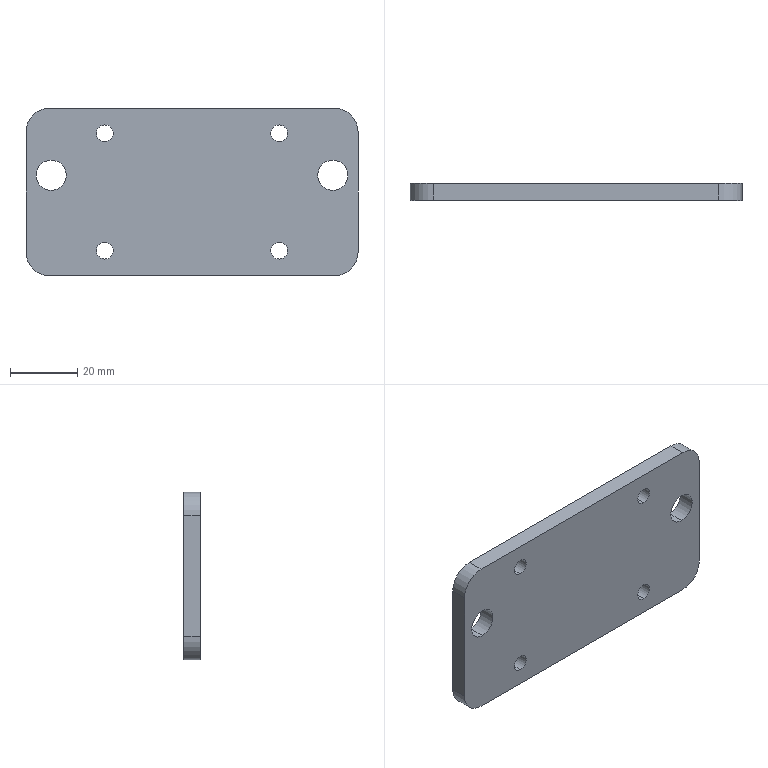Part | STEP file | 1.6米脚轮垫块 | 1 solid | 22 faces | box 99 x 5 x 50 mm | volume 23511 mm3 | cylinder 16 | plane 6 | commonest cylinder face diameters 5 x8 9 x4 14 x4
STEP:
#1=CARTESIAN_POINT('',(91.5,5.,-15.5));
#2=VERTEX_POINT('',#1);
#3=CARTESIAN_POINT('',(91.5,5.,-24.5));
#4=VERTEX_POINT('',#3);
#5=CARTESIAN_POINT('',(91.5,5.,-20.));
#6=DIRECTION('',(0.,-1.,0.));
#7=DIRECTION('',(0.,0.,-1.));
#8=AXIS2_PLACEMENT_3D('',#5,#6,#7);
#9=CIRCLE('',#8,4.5);
#10=EDGE_CURVE('',#2,#4,#9,.T.);
#11=ORIENTED_EDGE('',*,*,#10,.F.);
#12=CARTESIAN_POINT('',(91.5,0.,-15.5));
#13=VERTEX_POINT('',#12);
#14=CARTESIAN_POINT('',(91.5,10.,-15.5));
#15=DIRECTION('',(0.,-1.,0.));
#16=VECTOR('',#15,1000.);
#17=LINE('',#14,#16);
#18=EDGE_CURVE('',#2,#13,#17,.T.);
#19=ORIENTED_EDGE('',*,*,#18,.T.);
#20=CARTESIAN_POINT('',(91.5,0.,-24.5));
#21=VERTEX_POINT('',#20);
#22=CARTESIAN_POINT('',(91.5,0.,-20.));
#23=DIRECTION('',(0.,-1.,0.));
#24=DIRECTION('',(0.,0.,-1.));
#25=AXIS2_PLACEMENT_3D('',#22,#23,#24);
#26=CIRCLE('',#25,4.5);
#27=EDGE_CURVE('',#13,#21,#26,.T.);
#28=ORIENTED_EDGE('',*,*,#27,.T.);
#29=CARTESIAN_POINT('',(91.5,10.,-24.5));
#30=DIRECTION('',(0.,-1.,0.));
#31=VECTOR('',#30,1000.);
#32=LINE('',#29,#31);
#33=EDGE_CURVE('',#4,#21,#32,.T.);
#34=ORIENTED_EDGE('',*,*,#33,.F.);
#35=EDGE_LOOP('',(#11,#19,#28,#34));
#36=FACE_OUTER_BOUND('',#35,.T.);
#37=CARTESIAN_POINT('',(91.5,10.,-20.));
#38=DIRECTION('',(0.,-1.,0.));
#39=DIRECTION('',(0.,0.,-1.));
#40=AXIS2_PLACEMENT_3D('',#37,#38,#39);
#41=CYLINDRICAL_SURFACE('',#40,4.5);
#42=ADVANCED_FACE('',(#36),#41,.F.);
#43=CARTESIAN_POINT('',(7.5,5.,-15.5));
#44=VERTEX_POINT('',#43);
#45=CARTESIAN_POINT('',(7.5,5.,-24.5));
#46=VERTEX_POINT('',#45);
#47=CARTESIAN_POINT('',(7.5,5.,-20.));
#48=DIRECTION('',(0.,-1.,0.));
#49=DIRECTION('',(0.,0.,-1.));
#50=AXIS2_PLACEMENT_3D('',#47,#48,#49);
#51=CIRCLE('',#50,4.5);
#52=EDGE_CURVE('',#44,#46,#51,.T.);
#53=ORIENTED_EDGE('',*,*,#52,.F.);
#54=CARTESIAN_POINT('',(7.5,0.,-15.5));
#55=VERTEX_POINT('',#54);
#56=CARTESIAN_POINT('',(7.5,10.,-15.5));
#57=DIRECTION('',(0.,-1.,0.));
#58=VECTOR('',#57,1000.);
#59=LINE('',#56,#58);
#60=EDGE_CURVE('',#44,#55,#59,.T.);
#61=ORIENTED_EDGE('',*,*,#60,.T.);
#62=CARTESIAN_POINT('',(7.5,0.,-24.5));
#63=VERTEX_POINT('',#62);
#64=CARTESIAN_POINT('',(7.5,0.,-20.));
#65=DIRECTION('',(0.,-1.,0.));
#66=DIRECTION('',(0.,0.,-1.));
#67=AXIS2_PLACEMENT_3D('',#64,#65,#66);
#68=CIRCLE('',#67,4.5);
#69=EDGE_CURVE('',#55,#63,#68,.T.);
#70=ORIENTED_EDGE('',*,*,#69,.T.);
#71=CARTESIAN_POINT('',(7.5,10.,-24.5));
#72=DIRECTION('',(0.,-1.,0.));
#73=VECTOR('',#72,1000.);
#74=LINE('',#71,#73);
#75=EDGE_CURVE('',#46,#63,#74,.T.);
#76=ORIENTED_EDGE('',*,*,#75,.F.);
#77=EDGE_LOOP('',(#53,#61,#70,#76));
#78=FACE_OUTER_BOUND('',#77,.T.);
#79=CARTESIAN_POINT('',(7.5,10.,-20.));
#80=DIRECTION('',(0.,-1.,0.));
#81=DIRECTION('',(0.,0.,-1.));
#82=AXIS2_PLACEMENT_3D('',#79,#80,#81);
#83=CYLINDRICAL_SURFACE('',#82,4.5);
#84=ADVANCED_FACE('',(#78),#83,.F.);
#85=CARTESIAN_POINT('',(75.5,5.,-40.));
#86=VERTEX_POINT('',#85);
#87=CARTESIAN_POINT('',(75.5,5.,-45.));
#88=VERTEX_POINT('',#87);
#89=CARTESIAN_POINT('',(75.5,5.,-42.5));
#90=DIRECTION('',(0.,-1.,0.));
#91=DIRECTION('',(0.,0.,-1.));
#92=AXIS2_PLACEMENT_3D('',#89,#90,#91);
#93=CIRCLE('',#92,2.5);
#94=EDGE_CURVE('',#86,#88,#93,.T.);
#95=ORIENTED_EDGE('',*,*,#94,.F.);
#96=CARTESIAN_POINT('',(75.5,0.,-40.));
#97=VERTEX_POINT('',#96);
#98=CARTESIAN_POINT('',(75.5,0.,-40.));
#99=DIRECTION('',(0.,-1.,0.));
#100=VECTOR('',#99,1000.);
#101=LINE('',#98,#100);
#102=EDGE_CURVE('',#86,#97,#101,.T.);
#103=ORIENTED_EDGE('',*,*,#102,.T.);
#104=CARTESIAN_POINT('',(75.5,0.,-45.));
#105=VERTEX_POINT('',#104);
#106=CARTESIAN_POINT('',(75.5,0.,-42.5));
#107=DIRECTION('',(0.,-1.,0.));
#108=DIRECTION('',(0.,0.,-1.));
#109=AXIS2_PLACEMENT_3D('',#106,#107,#108);
#110=CIRCLE('',#109,2.5);
#111=EDGE_CURVE('',#97,#105,#110,.T.);
#112=ORIENTED_EDGE('',*,*,#111,.T.);
#113=CARTESIAN_POINT('',(75.5,0.,-45.));
#114=DIRECTION('',(0.,-1.,0.));
#115=VECTOR('',#114,1000.);
#116=LINE('',#113,#115);
#117=EDGE_CURVE('',#88,#105,#116,.T.);
#118=ORIENTED_EDGE('',*,*,#117,.F.);
#119=EDGE_LOOP('',(#95,#103,#112,#118));
#120=FACE_OUTER_BOUND('',#119,.T.);
#121=CARTESIAN_POINT('',(75.5,0.,-42.5));
#122=DIRECTION('',(0.,-1.,0.));
#123=DIRECTION('',(0.,0.,-1.));
#124=AXIS2_PLACEMENT_3D('',#121,#122,#123);
#125=CYLINDRICAL_SURFACE('',#124,2.5);
#126=ADVANCED_FACE('',(#120),#125,.F.);
#127=CARTESIAN_POINT('',(23.5,5.,-40.));
#128=VERTEX_POINT('',#127);
#129=CARTESIAN_POINT('',(23.5,5.,-45.));
#130=VERTEX_POINT('',#129);
#131=CARTESIAN_POINT('',(23.5,5.,-42.5));
#132=DIRECTION('',(0.,-1.,0.));
#133=DIRECTION('',(0.,0.,-1.));
#134=AXIS2_PLACEMENT_3D('',#131,#132,#133);
#135=CIRCLE('',#134,2.5);
#136=EDGE_CURVE('',#128,#130,#135,.T.);
#137=ORIENTED_EDGE('',*,*,#136,.F.);
#138=CARTESIAN_POINT('',(23.5,0.,-40.));
#139=VERTEX_POINT('',#138);
#140=CARTESIAN_POINT('',(23.5,0.,-40.));
#141=DIRECTION('',(0.,-1.,0.));
#142=VECTOR('',#141,1000.);
#143=LINE('',#140,#142);
#144=EDGE_CURVE('',#128,#139,#143,.T.);
#145=ORIENTED_EDGE('',*,*,#144,.T.);
#146=CARTESIAN_POINT('',(23.5,0.,-45.));
#147=VERTEX_POINT('',#146);
#148=CARTESIAN_POINT('',(23.5,0.,-42.5));
#149=DIRECTION('',(0.,-1.,0.));
#150=DIRECTION('',(0.,0.,-1.));
#151=AXIS2_PLACEMENT_3D('',#148,#149,#150);
#152=CIRCLE('',#151,2.5);
#153=EDGE_CURVE('',#139,#147,#152,.T.);
#154=ORIENTED_EDGE('',*,*,#153,.T.);
#155=CARTESIAN_POINT('',(23.5,0.,-45.));
#156=DIRECTION('',(0.,-1.,0.));
#157=VECTOR('',#156,1000.);
#158=LINE('',#155,#157);
#159=EDGE_CURVE('',#130,#147,#158,.T.);
#160=ORIENTED_EDGE('',*,*,#159,.F.);
#161=EDGE_LOOP('',(#137,#145,#154,#160));
#162=FACE_OUTER_BOUND('',#161,.T.);
#163=CARTESIAN_POINT('',(23.5,0.,-42.5));
#164=DIRECTION('',(0.,-1.,0.));
#165=DIRECTION('',(0.,0.,-1.));
#166=AXIS2_PLACEMENT_3D('',#163,#164,#165);
#167=CYLINDRICAL_SURFACE('',#166,2.5);
#168=ADVANCED_FACE('',(#162),#167,.F.);
#169=CARTESIAN_POINT('',(75.5,5.,-5.));
#170=VERTEX_POINT('',#169);
#171=CARTESIAN_POINT('',(75.5,5.,-10.));
#172=VERTEX_POINT('',#171);
#173=CARTESIAN_POINT('',(75.5,5.,-7.5));
#174=DIRECTION('',(0.,-1.,0.));
#175=DIRECTION('',(0.,0.,-1.));
#176=AXIS2_PLACEMENT_3D('',#173,#174,#175);
#177=CIRCLE('',#176,2.5);
#178=EDGE_CURVE('',#170,#172,#177,.T.);
#179=ORIENTED_EDGE('',*,*,#178,.F.);
#180=CARTESIAN_POINT('',(75.5,0.,-5.));
#181=VERTEX_POINT('',#180);
#182=CARTESIAN_POINT('',(75.5,0.,-5.));
#183=DIRECTION('',(0.,-1.,0.));
#184=VECTOR('',#183,1000.);
#185=LINE('',#182,#184);
#186=EDGE_CURVE('',#170,#181,#185,.T.);
#187=ORIENTED_EDGE('',*,*,#186,.T.);
#188=CARTESIAN_POINT('',(75.5,0.,-10.));
#189=VERTEX_POINT('',#188);
#190=CARTESIAN_POINT('',(75.5,0.,-7.5));
#191=DIRECTION('',(0.,-1.,0.));
#192=DIRECTION('',(0.,0.,-1.));
#193=AXIS2_PLACEMENT_3D('',#190,#191,#192);
#194=CIRCLE('',#193,2.5);
#195=EDGE_CURVE('',#181,#189,#194,.T.);
#196=ORIENTED_EDGE('',*,*,#195,.T.);
#197=CARTESIAN_POINT('',(75.5,0.,-10.));
#198=DIRECTION('',(0.,-1.,0.));
#199=VECTOR('',#198,1000.);
#200=LINE('',#197,#199);
#201=EDGE_CURVE('',#172,#189,#200,.T.);
#202=ORIENTED_EDGE('',*,*,#201,.F.);
#203=EDGE_LOOP('',(#179,#187,#196,#202));
#204=FACE_OUTER_BOUND('',#203,.T.);
#205=CARTESIAN_POINT('',(75.5,0.,-7.5));
#206=DIRECTION('',(0.,-1.,0.));
#207=DIRECTION('',(0.,0.,-1.));
#208=AXIS2_PLACEMENT_3D('',#205,#206,#207);
#209=CYLINDRICAL_SURFACE('',#208,2.5);
#210=ADVANCED_FACE('',(#204),#209,.F.);
#211=CARTESIAN_POINT('',(23.5,5.,-5.));
#212=VERTEX_POINT('',#211);
#213=CARTESIAN_POINT('',(23.5,5.,-10.));
#214=VERTEX_POINT('',#213);
#215=CARTESIAN_POINT('',(23.5,5.,-7.5));
#216=DIRECTION('',(0.,-1.,0.));
#217=DIRECTION('',(0.,0.,-1.));
#218=AXIS2_PLACEMENT_3D('',#215,#216,#217);
#219=CIRCLE('',#218,2.5);
#220=EDGE_CURVE('',#212,#214,#219,.T.);
#221=ORIENTED_EDGE('',*,*,#220,.F.);
#222=CARTESIAN_POINT('',(23.5,0.,-5.));
#223=VERTEX_POINT('',#222);
#224=CARTESIAN_POINT('',(23.5,0.,-5.));
#225=DIRECTION('',(0.,-1.,0.));
#226=VECTOR('',#225,1000.);
#227=LINE('',#224,#226);
#228=EDGE_CURVE('',#212,#223,#227,.T.);
#229=ORIENTED_EDGE('',*,*,#228,.T.);
#230=CARTESIAN_POINT('',(23.5,0.,-10.));
#231=VERTEX_POINT('',#230);
#232=CARTESIAN_POINT('',(23.5,0.,-7.5));
#233=DIRECTION('',(0.,-1.,0.));
#234=DIRECTION('',(0.,0.,-1.));
#235=AXIS2_PLACEMENT_3D('',#232,#233,#234);
#236=CIRCLE('',#235,2.5);
#237=EDGE_CURVE('',#223,#231,#236,.T.);
#238=ORIENTED_EDGE('',*,*,#237,.T.);
#239=CARTESIAN_POINT('',(23.5,0.,-10.));
#240=DIRECTION('',(0.,-1.,0.));
#241=VECTOR('',#240,1000.);
#242=LINE('',#239,#241);
#243=EDGE_CURVE('',#214,#231,#242,.T.);
#244=ORIENTED_EDGE('',*,*,#243,.F.);
#245=EDGE_LOOP('',(#221,#229,#238,#244));
#246=FACE_OUTER_BOUND('',#245,.T.);
#247=CARTESIAN_POINT('',(23.5,0.,-7.5));
#248=DIRECTION('',(0.,-1.,0.));
#249=DIRECTION('',(0.,0.,-1.));
#250=AXIS2_PLACEMENT_3D('',#247,#248,#249);
#251=CYLINDRICAL_SURFACE('',#250,2.5);
#252=ADVANCED_FACE('',(#246),#251,.F.);
#253=CARTESIAN_POINT('',(0.,5.,-43.));
#254=VERTEX_POINT('',#253);
#255=CARTESIAN_POINT('',(0.,5.,-7.));
#256=VERTEX_POINT('',#255);
#257=CARTESIAN_POINT('',(0.,5.,0.));
#258=DIRECTION('',(0.,0.,1.));
#259=VECTOR('',#258,1000.);
#260=LINE('',#257,#259);
#261=EDGE_CURVE('',#254,#256,#260,.T.);
#262=ORIENTED_EDGE('',*,*,#261,.F.);
#263=CARTESIAN_POINT('',(0.,0.,-43.));
#264=VERTEX_POINT('',#263);
#265=CARTESIAN_POINT('',(0.,5.,-43.));
#266=DIRECTION('',(0.,-1.,0.));
#267=VECTOR('',#266,1000.);
#268=LINE('',#265,#267);
#269=EDGE_CURVE('',#254,#264,#268,.T.);
#270=ORIENTED_EDGE('',*,*,#269,.T.);
#271=CARTESIAN_POINT('',(0.,0.,-7.));
#272=VERTEX_POINT('',#271);
#273=CARTESIAN_POINT('',(0.,0.,0.));
#274=DIRECTION('',(0.,0.,1.));
#275=VECTOR('',#274,1000.);
#276=LINE('',#273,#275);
#277=EDGE_CURVE('',#264,#272,#276,.T.);
#278=ORIENTED_EDGE('',*,*,#277,.T.);
#279=CARTESIAN_POINT('',(0.,5.,-7.));
#280=DIRECTION('',(0.,1.,0.));
#281=VECTOR('',#280,1000.);
#282=LINE('',#279,#281);
#283=EDGE_CURVE('',#272,#256,#282,.T.);
#284=ORIENTED_EDGE('',*,*,#283,.T.);
#285=EDGE_LOOP('',(#262,#270,#278,#284));
#286=FACE_OUTER_BOUND('',#285,.T.);
#287=CARTESIAN_POINT('',(0.,5.,0.));
#288=DIRECTION('',(1.,0.,0.));
#289=DIRECTION('',(0.,0.,-1.));
#290=AXIS2_PLACEMENT_3D('',#287,#288,#289);
#291=PLANE('',#290);
#292=ADVANCED_FACE('',(#286),#291,.F.);
#293=CARTESIAN_POINT('',(7.,0.,0.));
#294=VERTEX_POINT('',#293);
#295=CARTESIAN_POINT('',(92.,0.,0.));
#296=VERTEX_POINT('',#295);
#297=CARTESIAN_POINT('',(0.,0.,0.));
#298=DIRECTION('',(1.,0.,0.));
#299=VECTOR('',#298,1000.);
#300=LINE('',#297,#299);
#301=EDGE_CURVE('',#294,#296,#300,.T.);
#302=ORIENTED_EDGE('',*,*,#301,.T.);
#303=CARTESIAN_POINT('',(92.,5.,0.));
#304=VERTEX_POINT('',#303);
#305=CARTESIAN_POINT('',(92.,5.,0.));
#306=DIRECTION('',(0.,1.,0.));
#307=VECTOR('',#306,1000.);
#308=LINE('',#305,#307);
#309=EDGE_CURVE('',#296,#304,#308,.T.);
#310=ORIENTED_EDGE('',*,*,#309,.T.);
#311=CARTESIAN_POINT('',(7.,5.,0.));
#312=VERTEX_POINT('',#311);
#313=CARTESIAN_POINT('',(0.,5.,0.));
#314=DIRECTION('',(1.,0.,0.));
#315=VECTOR('',#314,1000.);
#316=LINE('',#313,#315);
#317=EDGE_CURVE('',#312,#304,#316,.T.);
#318=ORIENTED_EDGE('',*,*,#317,.F.);
#319=CARTESIAN_POINT('',(7.,5.,0.));
#320=DIRECTION('',(0.,-1.,0.));
#321=VECTOR('',#320,1000.);
#322=LINE('',#319,#321);
#323=EDGE_CURVE('',#312,#294,#322,.T.);
#324=ORIENTED_EDGE('',*,*,#323,.T.);
#325=EDGE_LOOP('',(#302,#310,#318,#324));
#326=FACE_OUTER_BOUND('',#325,.T.);
#327=CARTESIAN_POINT('',(0.,5.,0.));
#328=DIRECTION('',(0.,0.,-1.));
#329=DIRECTION('',(-1.,0.,0.));
#330=AXIS2_PLACEMENT_3D('',#327,#328,#329);
#331=PLANE('',#330);
#332=ADVANCED_FACE('',(#326),#331,.F.);
#333=CARTESIAN_POINT('',(99.,0.,-7.));
#334=VERTEX_POINT('',#333);
#335=CARTESIAN_POINT('',(99.,0.,-43.));
#336=VERTEX_POINT('',#335);
#337=CARTESIAN_POINT('',(99.,0.,0.));
#338=DIRECTION('',(0.,0.,-1.));
#339=VECTOR('',#338,1000.);
#340=LINE('',#337,#339);
#341=EDGE_CURVE('',#334,#336,#340,.T.);
#342=ORIENTED_EDGE('',*,*,#341,.T.);
#343=CARTESIAN_POINT('',(99.,5.,-43.));
#344=VERTEX_POINT('',#343);
#345=CARTESIAN_POINT('',(99.,5.,-43.));
#346=DIRECTION('',(0.,1.,0.));
#347=VECTOR('',#346,1000.);
#348=LINE('',#345,#347);
#349=EDGE_CURVE('',#336,#344,#348,.T.);
#350=ORIENTED_EDGE('',*,*,#349,.T.);
#351=CARTESIAN_POINT('',(99.,5.,-7.));
#352=VERTEX_POINT('',#351);
#353=CARTESIAN_POINT('',(99.,5.,0.));
#354=DIRECTION('',(0.,0.,-1.));
#355=VECTOR('',#354,1000.);
#356=LINE('',#353,#355);
#357=EDGE_CURVE('',#352,#344,#356,.T.);
#358=ORIENTED_EDGE('',*,*,#357,.F.);
#359=CARTESIAN_POINT('',(99.,5.,-7.));
#360=DIRECTION('',(0.,-1.,0.));
#361=VECTOR('',#360,1000.);
#362=LINE('',#359,#361);
#363=EDGE_CURVE('',#352,#334,#362,.T.);
#364=ORIENTED_EDGE('',*,*,#363,.T.);
#365=EDGE_LOOP('',(#342,#350,#358,#364));
#366=FACE_OUTER_BOUND('',#365,.T.);
#367=CARTESIAN_POINT('',(99.,5.,0.));
#368=DIRECTION('',(-1.,0.,0.));
#369=DIRECTION('',(0.,0.,1.));
#370=AXIS2_PLACEMENT_3D('',#367,#368,#369);
#371=PLANE('',#370);
#372=ADVANCED_FACE('',(#366),#371,.F.);
#373=CARTESIAN_POINT('',(92.,0.,-50.));
#374=VERTEX_POINT('',#373);
#375=CARTESIAN_POINT('',(7.,0.,-50.));
#376=VERTEX_POINT('',#375);
#377=CARTESIAN_POINT('',(0.,0.,-50.));
#378=DIRECTION('',(-1.,0.,0.));
#379=VECTOR('',#378,1000.);
#380=LINE('',#377,#379);
#381=EDGE_CURVE('',#374,#376,#380,.T.);
#382=ORIENTED_EDGE('',*,*,#381,.T.);
#383=CARTESIAN_POINT('',(7.,5.,-50.));
#384=VERTEX_POINT('',#383);
#385=CARTESIAN_POINT('',(7.,5.,-50.));
#386=DIRECTION('',(0.,1.,0.));
#387=VECTOR('',#386,1000.);
#388=LINE('',#385,#387);
#389=EDGE_CURVE('',#376,#384,#388,.T.);
#390=ORIENTED_EDGE('',*,*,#389,.T.);
#391=CARTESIAN_POINT('',(92.,5.,-50.));
#392=VERTEX_POINT('',#391);
#393=CARTESIAN_POINT('',(0.,5.,-50.));
#394=DIRECTION('',(-1.,0.,0.));
#395=VECTOR('',#394,1000.);
#396=LINE('',#393,#395);
#397=EDGE_CURVE('',#392,#384,#396,.T.);
#398=ORIENTED_EDGE('',*,*,#397,.F.);
#399=CARTESIAN_POINT('',(92.,5.,-50.));
#400=DIRECTION('',(0.,-1.,0.));
#401=VECTOR('',#400,1000.);
#402=LINE('',#399,#401);
#403=EDGE_CURVE('',#392,#374,#402,.T.);
#404=ORIENTED_EDGE('',*,*,#403,.T.);
#405=EDGE_LOOP('',(#382,#390,#398,#404));
#406=FACE_OUTER_BOUND('',#405,.T.);
#407=CARTESIAN_POINT('',(0.,5.,-50.));
#408=DIRECTION('',(0.,0.,1.));
#409=DIRECTION('',(1.,0.,0.));
#410=AXIS2_PLACEMENT_3D('',#407,#408,#409);
#411=PLANE('',#410);
#412=ADVANCED_FACE('',(#406),#411,.F.);
#413=CARTESIAN_POINT('',(91.5,5.,-20.));
#414=DIRECTION('',(0.,-1.,0.));
#415=DIRECTION('',(0.,0.,-1.));
#416=AXIS2_PLACEMENT_3D('',#413,#414,#415);
#417=CIRCLE('',#416,4.5);
#418=EDGE_CURVE('',#4,#2,#417,.T.);
#419=ORIENTED_EDGE('',*,*,#418,.T.);
#420=ORIENTED_EDGE('',*,*,#10,.T.);
#421=EDGE_LOOP('',(#419,#420));
#422=FACE_BOUND('',#421,.T.);
#423=CARTESIAN_POINT('',(7.5,5.,-20.));
#424=DIRECTION('',(0.,-1.,0.));
#425=DIRECTION('',(0.,0.,-1.));
#426=AXIS2_PLACEMENT_3D('',#423,#424,#425);
#427=CIRCLE('',#426,4.5);
#428=EDGE_CURVE('',#46,#44,#427,.T.);
#429=ORIENTED_EDGE('',*,*,#428,.T.);
#430=ORIENTED_EDGE('',*,*,#52,.T.);
#431=EDGE_LOOP('',(#429,#430));
#432=FACE_BOUND('',#431,.T.);
#433=CARTESIAN_POINT('',(75.5,5.,-42.5));
#434=DIRECTION('',(0.,-1.,0.));
#435=DIRECTION('',(0.,0.,-1.));
#436=AXIS2_PLACEMENT_3D('',#433,#434,#435);
#437=CIRCLE('',#436,2.5);
#438=EDGE_CURVE('',#88,#86,#437,.T.);
#439=ORIENTED_EDGE('',*,*,#438,.T.);
#440=ORIENTED_EDGE('',*,*,#94,.T.);
#441=EDGE_LOOP('',(#439,#440));
#442=FACE_BOUND('',#441,.T.);
#443=CARTESIAN_POINT('',(23.5,5.,-42.5));
#444=DIRECTION('',(0.,-1.,0.));
#445=DIRECTION('',(0.,0.,-1.));
#446=AXIS2_PLACEMENT_3D('',#443,#444,#445);
#447=CIRCLE('',#446,2.5);
#448=EDGE_CURVE('',#130,#128,#447,.T.);
#449=ORIENTED_EDGE('',*,*,#448,.T.);
#450=ORIENTED_EDGE('',*,*,#136,.T.);
#451=EDGE_LOOP('',(#449,#450));
#452=FACE_BOUND('',#451,.T.);
#453=CARTESIAN_POINT('',(75.5,5.,-7.5));
#454=DIRECTION('',(0.,-1.,0.));
#455=DIRECTION('',(0.,0.,-1.));
#456=AXIS2_PLACEMENT_3D('',#453,#454,#455);
#457=CIRCLE('',#456,2.5);
#458=EDGE_CURVE('',#172,#170,#457,.T.);
#459=ORIENTED_EDGE('',*,*,#458,.T.);
#460=ORIENTED_EDGE('',*,*,#178,.T.);
#461=EDGE_LOOP('',(#459,#460));
#462=FACE_BOUND('',#461,.T.);
#463=CARTESIAN_POINT('',(23.5,5.,-7.5));
#464=DIRECTION('',(0.,-1.,0.));
#465=DIRECTION('',(0.,0.,-1.));
#466=AXIS2_PLACEMENT_3D('',#463,#464,#465);
#467=CIRCLE('',#466,2.5);
#468=EDGE_CURVE('',#214,#212,#467,.T.);
#469=ORIENTED_EDGE('',*,*,#468,.T.);
#470=ORIENTED_EDGE('',*,*,#220,.T.);
#471=EDGE_LOOP('',(#469,#470));
#472=FACE_BOUND('',#471,.T.);
#473=ORIENTED_EDGE('',*,*,#397,.T.);
#474=CARTESIAN_POINT('',(7.,5.,-43.));
#475=DIRECTION('',(0.,1.,0.));
#476=DIRECTION('',(0.,0.,-1.));
#477=AXIS2_PLACEMENT_3D('',#474,#475,#476);
#478=CIRCLE('',#477,7.);
#479=EDGE_CURVE('',#384,#254,#478,.T.);
#480=ORIENTED_EDGE('',*,*,#479,.T.);
#481=ORIENTED_EDGE('',*,*,#261,.T.);
#482=CARTESIAN_POINT('',(7.,5.,-7.));
#483=DIRECTION('',(0.,1.,0.));
#484=DIRECTION('',(0.,0.,-1.));
#485=AXIS2_PLACEMENT_3D('',#482,#483,#484);
#486=CIRCLE('',#485,7.);
#487=EDGE_CURVE('',#256,#312,#486,.T.);
#488=ORIENTED_EDGE('',*,*,#487,.T.);
#489=ORIENTED_EDGE('',*,*,#317,.T.);
#490=CARTESIAN_POINT('',(92.,5.,-7.));
#491=DIRECTION('',(0.,1.,0.));
#492=DIRECTION('',(0.,0.,-1.));
#493=AXIS2_PLACEMENT_3D('',#490,#491,#492);
#494=CIRCLE('',#493,7.);
#495=EDGE_CURVE('',#304,#352,#494,.T.);
#496=ORIENTED_EDGE('',*,*,#495,.T.);
#497=ORIENTED_EDGE('',*,*,#357,.T.);
#498=CARTESIAN_POINT('',(92.,5.,-43.));
#499=DIRECTION('',(0.,1.,0.));
#500=DIRECTION('',(0.,0.,-1.));
#501=AXIS2_PLACEMENT_3D('',#498,#499,#500);
#502=CIRCLE('',#501,7.);
#503=EDGE_CURVE('',#344,#392,#502,.T.);
#504=ORIENTED_EDGE('',*,*,#503,.T.);
#505=EDGE_LOOP('',(#473,#480,#481,#488,#489,#496,#497,#504));
#506=FACE_OUTER_BOUND('',#505,.T.);
#507=CARTESIAN_POINT('',(0.,5.,0.));
#508=DIRECTION('',(0.,-1.,0.));
#509=DIRECTION('',(0.,0.,-1.));
#510=AXIS2_PLACEMENT_3D('',#507,#508,#509);
#511=PLANE('',#510);
#512=ADVANCED_FACE('',(#422,#432,#442,#452,#462,#472,#506),#511,.F.);
#513=CARTESIAN_POINT('',(91.5,0.,-20.));
#514=DIRECTION('',(0.,-1.,0.));
#515=DIRECTION('',(0.,0.,-1.));
#516=AXIS2_PLACEMENT_3D('',#513,#514,#515);
#517=CIRCLE('',#516,4.5);
#518=EDGE_CURVE('',#21,#13,#517,.T.);
#519=ORIENTED_EDGE('',*,*,#518,.F.);
#520=ORIENTED_EDGE('',*,*,#27,.F.);
#521=EDGE_LOOP('',(#519,#520));
#522=FACE_BOUND('',#521,.T.);
#523=CARTESIAN_POINT('',(7.5,0.,-20.));
#524=DIRECTION('',(0.,-1.,0.));
#525=DIRECTION('',(0.,0.,-1.));
#526=AXIS2_PLACEMENT_3D('',#523,#524,#525);
#527=CIRCLE('',#526,4.5);
#528=EDGE_CURVE('',#63,#55,#527,.T.);
#529=ORIENTED_EDGE('',*,*,#528,.F.);
#530=ORIENTED_EDGE('',*,*,#69,.F.);
#531=EDGE_LOOP('',(#529,#530));
#532=FACE_BOUND('',#531,.T.);
#533=CARTESIAN_POINT('',(75.5,0.,-42.5));
#534=DIRECTION('',(0.,-1.,0.));
#535=DIRECTION('',(0.,0.,-1.));
#536=AXIS2_PLACEMENT_3D('',#533,#534,#535);
#537=CIRCLE('',#536,2.5);
#538=EDGE_CURVE('',#105,#97,#537,.T.);
#539=ORIENTED_EDGE('',*,*,#538,.F.);
#540=ORIENTED_EDGE('',*,*,#111,.F.);
#541=EDGE_LOOP('',(#539,#540));
#542=FACE_BOUND('',#541,.T.);
#543=CARTESIAN_POINT('',(23.5,0.,-42.5));
#544=DIRECTION('',(0.,-1.,0.));
#545=DIRECTION('',(0.,0.,-1.));
#546=AXIS2_PLACEMENT_3D('',#543,#544,#545);
#547=CIRCLE('',#546,2.5);
#548=EDGE_CURVE('',#147,#139,#547,.T.);
#549=ORIENTED_EDGE('',*,*,#548,.F.);
#550=ORIENTED_EDGE('',*,*,#153,.F.);
#551=EDGE_LOOP('',(#549,#550));
#552=FACE_BOUND('',#551,.T.);
#553=CARTESIAN_POINT('',(75.5,0.,-7.5));
#554=DIRECTION('',(0.,-1.,0.));
#555=DIRECTION('',(0.,0.,-1.));
#556=AXIS2_PLACEMENT_3D('',#553,#554,#555);
#557=CIRCLE('',#556,2.5);
#558=EDGE_CURVE('',#189,#181,#557,.T.);
#559=ORIENTED_EDGE('',*,*,#558,.F.);
#560=ORIENTED_EDGE('',*,*,#195,.F.);
#561=EDGE_LOOP('',(#559,#560));
#562=FACE_BOUND('',#561,.T.);
#563=CARTESIAN_POINT('',(23.5,0.,-7.5));
#564=DIRECTION('',(0.,-1.,0.));
#565=DIRECTION('',(0.,0.,-1.));
#566=AXIS2_PLACEMENT_3D('',#563,#564,#565);
#567=CIRCLE('',#566,2.5);
#568=EDGE_CURVE('',#231,#223,#567,.T.);
#569=ORIENTED_EDGE('',*,*,#568,.F.);
#570=ORIENTED_EDGE('',*,*,#237,.F.);
#571=EDGE_LOOP('',(#569,#570));
#572=FACE_BOUND('',#571,.T.);
#573=ORIENTED_EDGE('',*,*,#277,.F.);
#574=CARTESIAN_POINT('',(7.,0.,-43.));
#575=DIRECTION('',(0.,-1.,0.));
#576=DIRECTION('',(0.,0.,-1.));
#577=AXIS2_PLACEMENT_3D('',#574,#575,#576);
#578=CIRCLE('',#577,7.);
#579=EDGE_CURVE('',#264,#376,#578,.T.);
#580=ORIENTED_EDGE('',*,*,#579,.T.);
#581=ORIENTED_EDGE('',*,*,#381,.F.);
#582=CARTESIAN_POINT('',(92.,0.,-43.));
#583=DIRECTION('',(0.,-1.,0.));
#584=DIRECTION('',(0.,0.,-1.));
#585=AXIS2_PLACEMENT_3D('',#582,#583,#584);
#586=CIRCLE('',#585,7.);
#587=EDGE_CURVE('',#374,#336,#586,.T.);
#588=ORIENTED_EDGE('',*,*,#587,.T.);
#589=ORIENTED_EDGE('',*,*,#341,.F.);
#590=CARTESIAN_POINT('',(92.,0.,-7.));
#591=DIRECTION('',(0.,-1.,0.));
#592=DIRECTION('',(0.,0.,-1.));
#593=AXIS2_PLACEMENT_3D('',#590,#591,#592);
#594=CIRCLE('',#593,7.);
#595=EDGE_CURVE('',#334,#296,#594,.T.);
#596=ORIENTED_EDGE('',*,*,#595,.T.);
#597=ORIENTED_EDGE('',*,*,#301,.F.);
#598=CARTESIAN_POINT('',(7.,0.,-7.));
#599=DIRECTION('',(0.,-1.,0.));
#600=DIRECTION('',(0.,0.,-1.));
#601=AXIS2_PLACEMENT_3D('',#598,#599,#600);
#602=CIRCLE('',#601,7.);
#603=EDGE_CURVE('',#294,#272,#602,.T.);
#604=ORIENTED_EDGE('',*,*,#603,.T.);
#605=EDGE_LOOP('',(#573,#580,#581,#588,#589,#596,#597,#604));
#606=FACE_OUTER_BOUND('',#605,.T.);
#607=CARTESIAN_POINT('',(0.,0.,0.));
#608=DIRECTION('',(0.,-1.,0.));
#609=DIRECTION('',(0.,0.,-1.));
#610=AXIS2_PLACEMENT_3D('',#607,#608,#609);
#611=PLANE('',#610);
#612=ADVANCED_FACE('',(#522,#532,#542,#552,#562,#572,#606),#611,.T.);
#613=ORIENTED_EDGE('',*,*,#479,.F.);
#614=ORIENTED_EDGE('',*,*,#389,.F.);
#615=ORIENTED_EDGE('',*,*,#579,.F.);
#616=ORIENTED_EDGE('',*,*,#269,.F.);
#617=EDGE_LOOP('',(#613,#614,#615,#616));
#618=FACE_OUTER_BOUND('',#617,.T.);
#619=CARTESIAN_POINT('',(7.,5.,-43.));
#620=DIRECTION('',(0.,-1.,0.));
#621=DIRECTION('',(0.,0.,-1.));
#622=AXIS2_PLACEMENT_3D('',#619,#620,#621);
#623=CYLINDRICAL_SURFACE('',#622,7.);
#624=ADVANCED_FACE('',(#618),#623,.T.);
#625=ORIENTED_EDGE('',*,*,#503,.F.);
#626=ORIENTED_EDGE('',*,*,#349,.F.);
#627=ORIENTED_EDGE('',*,*,#587,.F.);
#628=ORIENTED_EDGE('',*,*,#403,.F.);
#629=EDGE_LOOP('',(#625,#626,#627,#628));
#630=FACE_OUTER_BOUND('',#629,.T.);
#631=CARTESIAN_POINT('',(92.,5.,-43.));
#632=DIRECTION('',(0.,-1.,0.));
#633=DIRECTION('',(0.,0.,-1.));
#634=AXIS2_PLACEMENT_3D('',#631,#632,#633);
#635=CYLINDRICAL_SURFACE('',#634,7.);
#636=ADVANCED_FACE('',(#630),#635,.T.);
#637=ORIENTED_EDGE('',*,*,#495,.F.);
#638=ORIENTED_EDGE('',*,*,#309,.F.);
#639=ORIENTED_EDGE('',*,*,#595,.F.);
#640=ORIENTED_EDGE('',*,*,#363,.F.);
#641=EDGE_LOOP('',(#637,#638,#639,#640));
#642=FACE_OUTER_BOUND('',#641,.T.);
#643=CARTESIAN_POINT('',(92.,5.,-7.));
#644=DIRECTION('',(0.,-1.,0.));
#645=DIRECTION('',(0.,0.,-1.));
#646=AXIS2_PLACEMENT_3D('',#643,#644,#645);
#647=CYLINDRICAL_SURFACE('',#646,7.);
#648=ADVANCED_FACE('',(#642),#647,.T.);
#649=ORIENTED_EDGE('',*,*,#487,.F.);
#650=ORIENTED_EDGE('',*,*,#283,.F.);
#651=ORIENTED_EDGE('',*,*,#603,.F.);
#652=ORIENTED_EDGE('',*,*,#323,.F.);
#653=EDGE_LOOP('',(#649,#650,#651,#652));
#654=FACE_OUTER_BOUND('',#653,.T.);
#655=CARTESIAN_POINT('',(7.,5.,-7.));
#656=DIRECTION('',(0.,-1.,0.));
#657=DIRECTION('',(0.,0.,-1.));
#658=AXIS2_PLACEMENT_3D('',#655,#656,#657);
#659=CYLINDRICAL_SURFACE('',#658,7.);
#660=ADVANCED_FACE('',(#654),#659,.T.);
#661=ORIENTED_EDGE('',*,*,#228,.F.);
#662=ORIENTED_EDGE('',*,*,#468,.F.);
#663=ORIENTED_EDGE('',*,*,#243,.T.);
#664=ORIENTED_EDGE('',*,*,#568,.T.);
#665=EDGE_LOOP('',(#661,#662,#663,#664));
#666=FACE_OUTER_BOUND('',#665,.T.);
#667=CARTESIAN_POINT('',(23.5,0.,-7.5));
#668=DIRECTION('',(0.,-1.,0.));
#669=DIRECTION('',(0.,0.,-1.));
#670=AXIS2_PLACEMENT_3D('',#667,#668,#669);
#671=CYLINDRICAL_SURFACE('',#670,2.5);
#672=ADVANCED_FACE('',(#666),#671,.F.);
#673=ORIENTED_EDGE('',*,*,#186,.F.);
#674=ORIENTED_EDGE('',*,*,#458,.F.);
#675=ORIENTED_EDGE('',*,*,#201,.T.);
#676=ORIENTED_EDGE('',*,*,#558,.T.);
#677=EDGE_LOOP('',(#673,#674,#675,#676));
#678=FACE_OUTER_BOUND('',#677,.T.);
#679=CARTESIAN_POINT('',(75.5,0.,-7.5));
#680=DIRECTION('',(0.,-1.,0.));
#681=DIRECTION('',(0.,0.,-1.));
#682=AXIS2_PLACEMENT_3D('',#679,#680,#681);
#683=CYLINDRICAL_SURFACE('',#682,2.5);
#684=ADVANCED_FACE('',(#678),#683,.F.);
#685=ORIENTED_EDGE('',*,*,#144,.F.);
#686=ORIENTED_EDGE('',*,*,#448,.F.);
#687=ORIENTED_EDGE('',*,*,#159,.T.);
#688=ORIENTED_EDGE('',*,*,#548,.T.);
#689=EDGE_LOOP('',(#685,#686,#687,#688));
#690=FACE_OUTER_BOUND('',#689,.T.);
#691=CARTESIAN_POINT('',(23.5,0.,-42.5));
#692=DIRECTION('',(0.,-1.,0.));
#693=DIRECTION('',(0.,0.,-1.));
#694=AXIS2_PLACEMENT_3D('',#691,#692,#693);
#695=CYLINDRICAL_SURFACE('',#694,2.5);
#696=ADVANCED_FACE('',(#690),#695,.F.);
#697=ORIENTED_EDGE('',*,*,#102,.F.);
#698=ORIENTED_EDGE('',*,*,#438,.F.);
#699=ORIENTED_EDGE('',*,*,#117,.T.);
#700=ORIENTED_EDGE('',*,*,#538,.T.);
#701=EDGE_LOOP('',(#697,#698,#699,#700));
#702=FACE_OUTER_BOUND('',#701,.T.);
#703=CARTESIAN_POINT('',(75.5,0.,-42.5));
#704=DIRECTION('',(0.,-1.,0.));
#705=DIRECTION('',(0.,0.,-1.));
#706=AXIS2_PLACEMENT_3D('',#703,#704,#705);
#707=CYLINDRICAL_SURFACE('',#706,2.5);
#708=ADVANCED_FACE('',(#702),#707,.F.);
#709=ORIENTED_EDGE('',*,*,#60,.F.);
#710=ORIENTED_EDGE('',*,*,#428,.F.);
#711=ORIENTED_EDGE('',*,*,#75,.T.);
#712=ORIENTED_EDGE('',*,*,#528,.T.);
#713=EDGE_LOOP('',(#709,#710,#711,#712));
#714=FACE_OUTER_BOUND('',#713,.T.);
#715=CARTESIAN_POINT('',(7.5,10.,-20.));
#716=DIRECTION('',(0.,-1.,0.));
#717=DIRECTION('',(0.,0.,-1.));
#718=AXIS2_PLACEMENT_3D('',#715,#716,#717);
#719=CYLINDRICAL_SURFACE('',#718,4.5);
#720=ADVANCED_FACE('',(#714),#719,.F.);
#721=ORIENTED_EDGE('',*,*,#18,.F.);
#722=ORIENTED_EDGE('',*,*,#418,.F.);
#723=ORIENTED_EDGE('',*,*,#33,.T.);
#724=ORIENTED_EDGE('',*,*,#518,.T.);
#725=EDGE_LOOP('',(#721,#722,#723,#724));
#726=FACE_OUTER_BOUND('',#725,.T.);
#727=CARTESIAN_POINT('',(91.5,10.,-20.));
#728=DIRECTION('',(0.,-1.,0.));
#729=DIRECTION('',(0.,0.,-1.));
#730=AXIS2_PLACEMENT_3D('',#727,#728,#729);
#731=CYLINDRICAL_SURFACE('',#730,4.5);
#732=ADVANCED_FACE('',(#726),#731,.F.);
#733=CLOSED_SHELL('',(#42,#84,#126,#168,#210,#252,#292,#332,#372,#412,#512,#612,#624,#636,#648,#660,#672,#684,#696,#708,#720,#732));
#734=MANIFOLD_SOLID_BREP('',#733);
#735=CARTESIAN_POINT('',(0.,0.,0.));
#736=DIRECTION('',(0.,0.,1.));
#737=DIRECTION('',(1.,0.,0.));
#738=AXIS2_PLACEMENT_3D('',#735,#736,#737);
#739=(LENGTH_UNIT()NAMED_UNIT(*)SI_UNIT(.MILLI.,.METRE.));
#740=UNCERTAINTY_MEASURE_WITH_UNIT(LENGTH_MEASURE(0.00001),#739,'','');
#741=(NAMED_UNIT(*)PLANE_ANGLE_UNIT()SI_UNIT($,.RADIAN.));
#742=(NAMED_UNIT(*)SI_UNIT($,.STERADIAN.)SOLID_ANGLE_UNIT());
#743=(GEOMETRIC_REPRESENTATION_CONTEXT(3)GLOBAL_UNCERTAINTY_ASSIGNED_CONTEXT((#740))GLOBAL_UNIT_ASSIGNED_CONTEXT((#739,#741,#742))REPRESENTATION_CONTEXT('',''));
#744=ADVANCED_BREP_SHAPE_REPRESENTATION('',(#734,#738),#743);